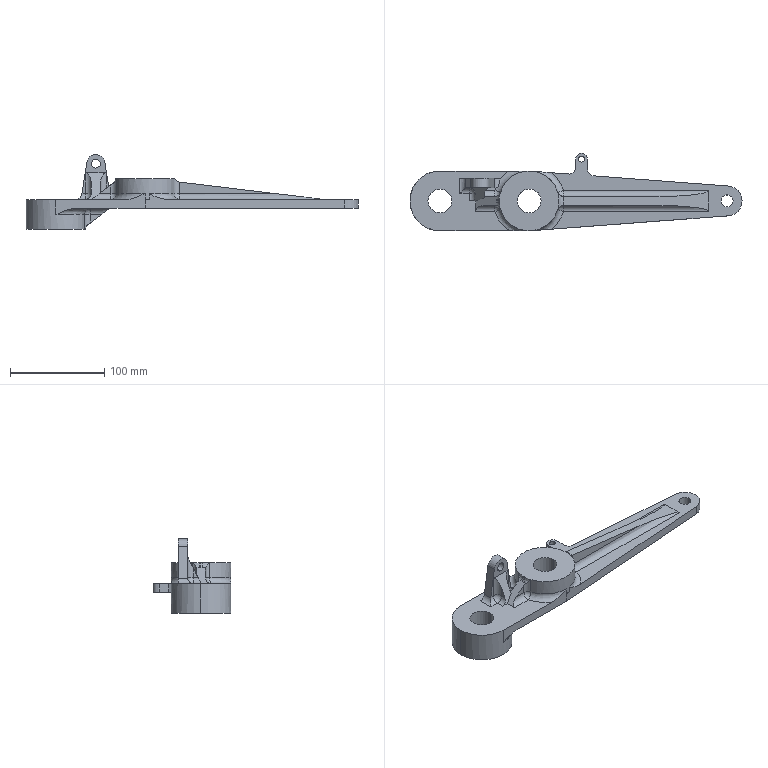Part | SolidWorks | features Fillet 9, ICE 4, Rib 4, Extrusion 1 | 1 solid | 92 faces | box 352.42 x 82.55 x 79.56 mm | volume 319205 mm3 | cylinder 40 | plane 31 | spline 8 | sphere 7 | torus 6 | commonest cylinder face diameters 12.7 x23 63.5 x7 25.4 x4 6.35 x2 9.525 x2 19.3 x1